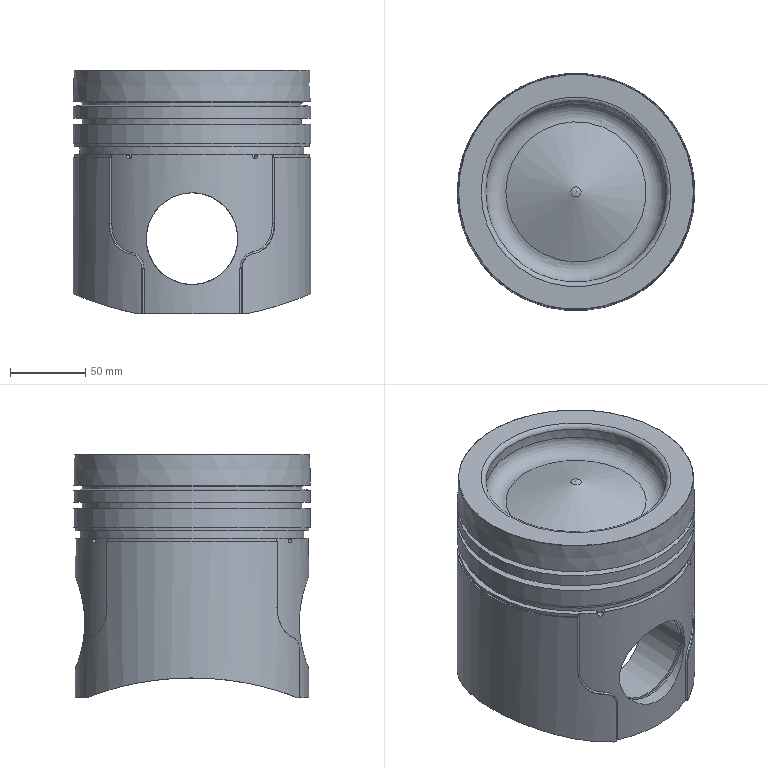Part | NX | features BLEND 23, EXTRUDE 12, DATUM_CSYS 11, SKETCH 10, HOLE PACKAGE 4, TAPER_HOLE 4, MIRROR_SET 3, SWP104 2, CHAMFER 1, CPROJ 1, DATUM_PLANE 1 | 1 solid | 157 faces | box 157.8 x 157.8 x 162 mm | volume 1466782 mm3 | cylinder 55 | spline 48 | plane 35 | cone 9 | torus 8 | sphere 2 | commonest cylinder face diameters 2 x16 10 x8 61 x4 157.8 x4 155.8 x3 20 x2